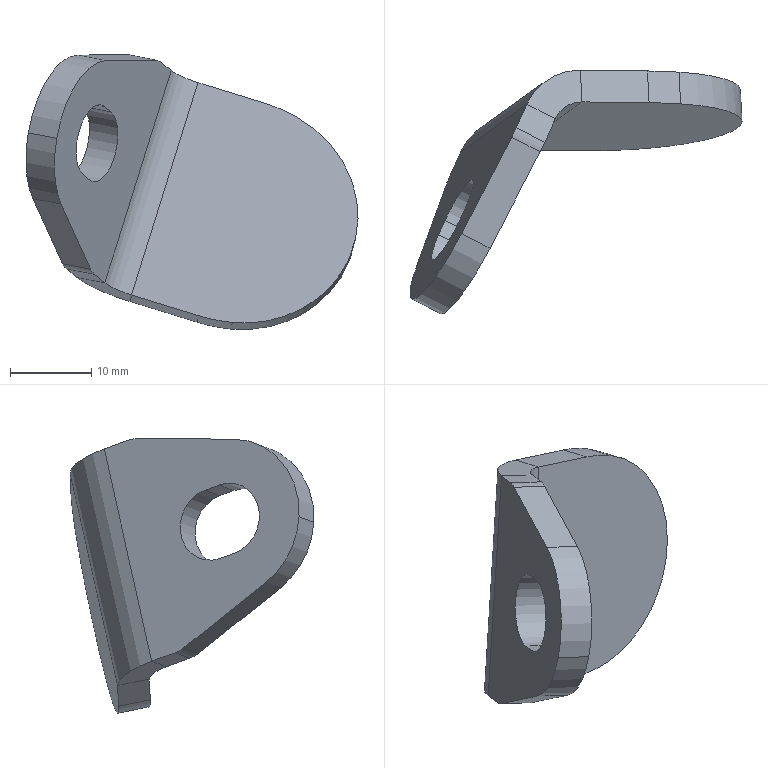Part | SolidWorks | features BaseBody 1 | 1 solid | 26 faces | box 40.878 x 30.009 x 33.842 mm | volume 4842 mm3 | plane 14 | cylinder 10 | spline 2 | commonest cylinder face diameters 8 x3 9 x2 20 x2 40 x2 16 x1
STEP:
#1=CARTESIAN_POINT('',(-7.748,15.098,8.963));
#2=VERTEX_POINT('',#1);
#3=CARTESIAN_POINT('',(-5.124,16.976,17.364));
#4=VERTEX_POINT('',#3);
#5=CARTESIAN_POINT('',(-6.436,16.037,13.163));
#6=DIRECTION('',(-0.8743,0.454,0.1717));
#7=DIRECTION('',(-0.2916,-0.2086,-0.9335));
#8=AXIS2_PLACEMENT_3D('',#5,#6,#7);
#9=CIRCLE('',#8,4.5);
#10=EDGE_CURVE('',#2,#4,#9,.T.);
#11=ORIENTED_EDGE('',*,*,#10,.F.);
#12=CARTESIAN_POINT('',(-6.972,16.831,8.333));
#13=VERTEX_POINT('',#12);
#14=CARTESIAN_POINT('',(-6.972,16.831,8.333));
#15=DIRECTION('',(-0.388,-0.8662,0.3148));
#16=VECTOR('',#15,1000.);
#17=LINE('',#14,#16);
#18=EDGE_CURVE('',#13,#2,#17,.T.);
#19=ORIENTED_EDGE('',*,*,#18,.F.);
#20=CARTESIAN_POINT('',(-4.348,18.709,16.734));
#21=VERTEX_POINT('',#20);
#22=CARTESIAN_POINT('',(-5.66,17.77,12.534));
#23=DIRECTION('',(-0.8743,0.454,0.1717));
#24=DIRECTION('',(0.2916,0.2086,0.9335));
#25=AXIS2_PLACEMENT_3D('',#22,#23,#24);
#26=CIRCLE('',#25,4.5);
#27=EDGE_CURVE('',#21,#13,#26,.T.);
#28=ORIENTED_EDGE('',*,*,#27,.F.);
#29=CARTESIAN_POINT('',(-5.124,16.976,17.364));
#30=DIRECTION('',(0.388,0.8662,-0.3148));
#31=VECTOR('',#30,1000.);
#32=LINE('',#29,#31);
#33=EDGE_CURVE('',#4,#21,#32,.T.);
#34=ORIENTED_EDGE('',*,*,#33,.F.);
#35=EDGE_LOOP('',(#11,#19,#28,#34));
#36=FACE_BOUND('',#35,.T.);
#37=CARTESIAN_POINT('',(3.098,31.128,21.809));
#38=VERTEX_POINT('',#37);
#39=CARTESIAN_POINT('',(1.803,28.238,22.859));
#40=VERTEX_POINT('',#39);
#41=CARTESIAN_POINT('',(3.098,31.128,21.809));
#42=DIRECTION('',(-0.388,-0.8662,0.3148));
#43=VECTOR('',#42,1000.);
#44=LINE('',#41,#43);
#45=EDGE_CURVE('',#38,#40,#44,.T.);
#46=ORIENTED_EDGE('',*,*,#45,.F.);
#47=CARTESIAN_POINT('',(-5.068,25.286,-4.329));
#48=VERTEX_POINT('',#47);
#49=CARTESIAN_POINT('',(-5.068,25.286,-4.329));
#50=DIRECTION('',(0.2916,0.2086,0.9335));
#51=VECTOR('',#50,1000.);
#52=LINE('',#49,#51);
#53=EDGE_CURVE('',#48,#38,#52,.T.);
#54=ORIENTED_EDGE('',*,*,#53,.F.);
#55=CARTESIAN_POINT('',(-6.362,22.396,-3.278));
#56=VERTEX_POINT('',#55);
#57=CARTESIAN_POINT('',(-6.362,22.396,-3.278));
#58=DIRECTION('',(0.388,0.8662,-0.3148));
#59=VECTOR('',#58,1000.);
#60=LINE('',#57,#59);
#61=EDGE_CURVE('',#56,#48,#60,.T.);
#62=ORIENTED_EDGE('',*,*,#61,.F.);
#63=CARTESIAN_POINT('',(-6.801,21.321,-2.671));
#64=VERTEX_POINT('',#63);
#65=CARTESIAN_POINT('',(-5.196,23.231,0.4555));
#66=DIRECTION('',(0.8743,-0.454,-0.1717));
#67=DIRECTION('',(-0.4014,-0.4775,-0.7816));
#68=AXIS2_PLACEMENT_3D('',#65,#66,#67);
#69=CIRCLE('',#68,4.);
#70=EDGE_CURVE('',#64,#56,#69,.T.);
#71=ORIENTED_EDGE('',*,*,#70,.F.);
#72=CARTESIAN_POINT('',(-10.45,11.263,5.347));
#73=VERTEX_POINT('',#72);
#74=CARTESIAN_POINT('',(-10.45,11.263,5.347));
#75=DIRECTION('',(0.2729,0.7523,-0.5997));
#76=VECTOR('',#75,1000.);
#77=LINE('',#74,#76);
#78=EDGE_CURVE('',#73,#64,#77,.T.);
#79=ORIENTED_EDGE('',*,*,#78,.F.);
#80=CARTESIAN_POINT('',(-10.998,7.143,13.448));
#81=VERTEX_POINT('',#80);
#82=CARTESIAN_POINT('',(-6.436,16.037,13.163));
#83=DIRECTION('',(0.8743,-0.454,-0.1717));
#84=DIRECTION('',(-0.4562,-0.8894,0.02851));
#85=AXIS2_PLACEMENT_3D('',#82,#83,#84);
#86=CIRCLE('',#85,10.);
#87=EDGE_CURVE('',#81,#73,#86,.T.);
#88=ORIENTED_EDGE('',*,*,#87,.F.);
#89=CARTESIAN_POINT('',(-4.93,15.211,23.015));
#90=VERTEX_POINT('',#89);
#91=CARTESIAN_POINT('',(-6.436,16.037,13.163));
#92=DIRECTION('',(0.8743,-0.454,-0.1717));
#93=DIRECTION('',(-0.4562,-0.8894,0.02851));
#94=AXIS2_PLACEMENT_3D('',#91,#92,#93);
#95=CIRCLE('',#94,10.);
#96=EDGE_CURVE('',#90,#81,#95,.T.);
#97=ORIENTED_EDGE('',*,*,#96,.F.);
#98=CARTESIAN_POINT('',(1.239,27.073,23.066));
#99=VERTEX_POINT('',#98);
#100=CARTESIAN_POINT('',(1.239,27.073,23.066));
#101=DIRECTION('',(-0.4614,-0.8872,-0.003841));
#102=VECTOR('',#101,1000.);
#103=LINE('',#100,#102);
#104=EDGE_CURVE('',#99,#90,#103,.T.);
#105=ORIENTED_EDGE('',*,*,#104,.F.);
#106=CARTESIAN_POINT('',(0.6369,27.404,19.125));
#107=DIRECTION('',(0.8743,-0.454,-0.1717));
#108=DIRECTION('',(0.2916,0.2086,0.9335));
#109=AXIS2_PLACEMENT_3D('',#106,#107,#108);
#110=CIRCLE('',#109,4.);
#111=EDGE_CURVE('',#40,#99,#110,.T.);
#112=ORIENTED_EDGE('',*,*,#111,.F.);
#113=EDGE_LOOP('',(#46,#54,#62,#71,#79,#88,#97,#105,#112));
#114=FACE_OUTER_BOUND('',#113,.T.);
#115=CARTESIAN_POINT('',(101.216,-68.081,783.905));
#116=DIRECTION('',(-0.8743,0.454,0.1717));
#117=DIRECTION('',(0.1927,0.,0.9813));
#118=AXIS2_PLACEMENT_3D('',#115,#116,#117);
#119=PLANE('',#118);
#120=ADVANCED_FACE('',(#36,#114),#119,.T.);
#121=CARTESIAN_POINT('',(5.301,26.422,22.173));
#122=VERTEX_POINT('',#121);
#123=CARTESIAN_POINT('',(1.803,28.238,22.859));
#124=DIRECTION('',(0.8743,-0.454,-0.1717));
#125=VECTOR('',#124,1000.);
#126=LINE('',#123,#125);
#127=EDGE_CURVE('',#40,#122,#126,.T.);
#128=ORIENTED_EDGE('',*,*,#127,.F.);
#129=ORIENTED_EDGE('',*,*,#111,.T.);
#130=CARTESIAN_POINT('',(4.736,25.257,22.379));
#131=VERTEX_POINT('',#130);
#132=CARTESIAN_POINT('',(4.736,25.257,22.379));
#133=DIRECTION('',(-0.8743,0.454,0.1717));
#134=VECTOR('',#133,1000.);
#135=LINE('',#132,#134);
#136=EDGE_CURVE('',#131,#99,#135,.T.);
#137=ORIENTED_EDGE('',*,*,#136,.F.);
#138=CARTESIAN_POINT('',(4.134,25.588,18.439));
#139=DIRECTION('',(-0.8743,0.454,0.1717));
#140=DIRECTION('',(0.1506,-0.08257,0.9851));
#141=AXIS2_PLACEMENT_3D('',#138,#139,#140);
#142=CIRCLE('',#141,4.);
#143=EDGE_CURVE('',#131,#122,#142,.T.);
#144=ORIENTED_EDGE('',*,*,#143,.T.);
#145=EDGE_LOOP('',(#128,#129,#137,#144));
#146=FACE_OUTER_BOUND('',#145,.T.);
#147=CARTESIAN_POINT('',(-83.852,71.275,35.714));
#148=DIRECTION('',(0.8743,-0.454,-0.1717));
#149=DIRECTION('',(0.2916,0.2086,0.9335));
#150=AXIS2_PLACEMENT_3D('',#147,#148,#149);
#151=CYLINDRICAL_SURFACE('',#150,4.);
#152=ADVANCED_FACE('',(#146),#151,.T.);
#153=CARTESIAN_POINT('',(-3.475,15.015,7.646));
#154=VERTEX_POINT('',#153);
#155=CARTESIAN_POINT('',(-0.8504,16.893,16.048));
#156=VERTEX_POINT('',#155);
#157=CARTESIAN_POINT('',(-2.163,15.954,11.847));
#158=DIRECTION('',(0.8743,-0.454,-0.1717));
#159=DIRECTION('',(-0.2916,-0.2086,-0.9335));
#160=AXIS2_PLACEMENT_3D('',#157,#158,#159);
#161=CIRCLE('',#160,4.5);
#162=EDGE_CURVE('',#154,#156,#161,.T.);
#163=ORIENTED_EDGE('',*,*,#162,.F.);
#164=CARTESIAN_POINT('',(-4.251,13.282,8.276));
#165=VERTEX_POINT('',#164);
#166=CARTESIAN_POINT('',(-4.251,13.282,8.276));
#167=DIRECTION('',(0.388,0.8662,-0.3148));
#168=VECTOR('',#167,1000.);
#169=LINE('',#166,#168);
#170=EDGE_CURVE('',#165,#154,#169,.T.);
#171=ORIENTED_EDGE('',*,*,#170,.F.);
#172=CARTESIAN_POINT('',(-1.626,15.16,16.677));
#173=VERTEX_POINT('',#172);
#174=CARTESIAN_POINT('',(-2.939,14.221,12.477));
#175=DIRECTION('',(0.8743,-0.454,-0.1717));
#176=DIRECTION('',(0.2916,0.2086,0.9335));
#177=AXIS2_PLACEMENT_3D('',#174,#175,#176);
#178=CIRCLE('',#177,4.5);
#179=EDGE_CURVE('',#173,#165,#178,.T.);
#180=ORIENTED_EDGE('',*,*,#179,.F.);
#181=CARTESIAN_POINT('',(-0.8504,16.893,16.048));
#182=DIRECTION('',(-0.388,-0.8662,0.3148));
#183=VECTOR('',#182,1000.);
#184=LINE('',#181,#183);
#185=EDGE_CURVE('',#156,#173,#184,.T.);
#186=ORIENTED_EDGE('',*,*,#185,.F.);
#187=EDGE_LOOP('',(#163,#171,#180,#186));
#188=FACE_BOUND('',#187,.T.);
#189=CARTESIAN_POINT('',(-1.433,13.396,22.328));
#190=VERTEX_POINT('',#189);
#191=CARTESIAN_POINT('',(-1.433,13.396,22.328));
#192=DIRECTION('',(0.4614,0.8872,0.003841));
#193=VECTOR('',#192,1000.);
#194=LINE('',#191,#193);
#195=EDGE_CURVE('',#190,#131,#194,.T.);
#196=ORIENTED_EDGE('',*,*,#195,.F.);
#197=CARTESIAN_POINT('',(-7.501,5.327,12.762));
#198=VERTEX_POINT('',#197);
#199=CARTESIAN_POINT('',(-2.939,14.221,12.477));
#200=DIRECTION('',(-0.8743,0.454,0.1717));
#201=DIRECTION('',(-0.4562,-0.8894,0.02851));
#202=AXIS2_PLACEMENT_3D('',#199,#200,#201);
#203=CIRCLE('',#202,10.);
#204=EDGE_CURVE('',#198,#190,#203,.T.);
#205=ORIENTED_EDGE('',*,*,#204,.F.);
#206=CARTESIAN_POINT('',(-6.953,9.447,4.66));
#207=VERTEX_POINT('',#206);
#208=CARTESIAN_POINT('',(-2.939,14.221,12.477));
#209=DIRECTION('',(-0.8743,0.454,0.1717));
#210=DIRECTION('',(-0.4562,-0.8894,0.02851));
#211=AXIS2_PLACEMENT_3D('',#208,#209,#210);
#212=CIRCLE('',#211,10.);
#213=EDGE_CURVE('',#207,#198,#212,.T.);
#214=ORIENTED_EDGE('',*,*,#213,.F.);
#215=CARTESIAN_POINT('',(-3.304,19.505,-3.358));
#216=VERTEX_POINT('',#215);
#217=CARTESIAN_POINT('',(-3.304,19.505,-3.358));
#218=DIRECTION('',(-0.2729,-0.7523,0.5997));
#219=VECTOR('',#218,1000.);
#220=LINE('',#217,#219);
#221=EDGE_CURVE('',#216,#207,#220,.T.);
#222=ORIENTED_EDGE('',*,*,#221,.F.);
#223=CARTESIAN_POINT('',(-2.865,20.58,-3.965));
#224=VERTEX_POINT('',#223);
#225=CARTESIAN_POINT('',(-1.698,21.415,-0.2311));
#226=DIRECTION('',(-0.8743,0.454,0.1717));
#227=DIRECTION('',(-0.2916,-0.2086,-0.9335));
#228=AXIS2_PLACEMENT_3D('',#225,#226,#227);
#229=CIRCLE('',#228,4.);
#230=EDGE_CURVE('',#224,#216,#229,.T.);
#231=ORIENTED_EDGE('',*,*,#230,.F.);
#232=CARTESIAN_POINT('',(-1.571,23.47,-5.015));
#233=VERTEX_POINT('',#232);
#234=CARTESIAN_POINT('',(-1.571,23.47,-5.015));
#235=DIRECTION('',(-0.388,-0.8662,0.3148));
#236=VECTOR('',#235,1000.);
#237=LINE('',#234,#236);
#238=EDGE_CURVE('',#233,#224,#237,.T.);
#239=ORIENTED_EDGE('',*,*,#238,.F.);
#240=CARTESIAN_POINT('',(6.595,29.312,21.123));
#241=VERTEX_POINT('',#240);
#242=CARTESIAN_POINT('',(6.595,29.312,21.123));
#243=DIRECTION('',(-0.2916,-0.2086,-0.9335));
#244=VECTOR('',#243,1000.);
#245=LINE('',#242,#244);
#246=EDGE_CURVE('',#241,#233,#245,.T.);
#247=ORIENTED_EDGE('',*,*,#246,.F.);
#248=CARTESIAN_POINT('',(5.301,26.422,22.173));
#249=DIRECTION('',(0.388,0.8662,-0.3148));
#250=VECTOR('',#249,1000.);
#251=LINE('',#248,#250);
#252=EDGE_CURVE('',#122,#241,#251,.T.);
#253=ORIENTED_EDGE('',*,*,#252,.F.);
#254=ORIENTED_EDGE('',*,*,#143,.F.);
#255=EDGE_LOOP('',(#196,#205,#214,#222,#231,#239,#247,#253,#254));
#256=FACE_OUTER_BOUND('',#255,.T.);
#257=CARTESIAN_POINT('',(104.713,-69.897,783.219));
#258=DIRECTION('',(-0.8743,0.454,0.1717));
#259=DIRECTION('',(0.1927,0.,0.9813));
#260=AXIS2_PLACEMENT_3D('',#257,#258,#259);
#261=PLANE('',#260);
#262=ADVANCED_FACE('',(#188,#256),#261,.F.);
#263=ORIENTED_EDGE('',*,*,#252,.T.);
#264=CARTESIAN_POINT('',(6.595,29.312,21.123));
#265=DIRECTION('',(-0.8743,0.454,0.1717));
#266=VECTOR('',#265,1000.);
#267=LINE('',#264,#266);
#268=EDGE_CURVE('',#241,#38,#267,.T.);
#269=ORIENTED_EDGE('',*,*,#268,.T.);
#270=ORIENTED_EDGE('',*,*,#45,.T.);
#271=ORIENTED_EDGE('',*,*,#127,.T.);
#272=EDGE_LOOP('',(#263,#269,#270,#271));
#273=FACE_OUTER_BOUND('',#272,.T.);
#274=CARTESIAN_POINT('',(-2.695,13.384,27.585));
#275=DIRECTION('',(-0.2916,-0.2086,-0.9335));
#276=DIRECTION('',(-0.9545,0.,0.2982));
#277=AXIS2_PLACEMENT_3D('',#274,#275,#276);
#278=PLANE('',#277);
#279=ADVANCED_FACE('',(#273),#278,.F.);
#280=ORIENTED_EDGE('',*,*,#268,.F.);
#281=CARTESIAN_POINT('',(9.887,31.408,19.626));
#282=VERTEX_POINT('',#281);
#283=CARTESIAN_POINT('',(10.092,27.496,20.436));
#284=DIRECTION('',(0.2916,0.2086,0.9335));
#285=DIRECTION('',(-0.05124,0.9779,-0.2026));
#286=AXIS2_PLACEMENT_3D('',#283,#284,#285);
#287=CIRCLE('',#286,4.);
#288=EDGE_CURVE('',#282,#241,#287,.T.);
#289=ORIENTED_EDGE('',*,*,#288,.F.);
#290=CARTESIAN_POINT('',(9.682,35.319,18.815));
#291=VERTEX_POINT('',#290);
#292=CARTESIAN_POINT('',(9.887,31.408,19.626));
#293=DIRECTION('',(-0.05124,0.9779,-0.2026));
#294=VECTOR('',#293,1000.);
#295=LINE('',#292,#294);
#296=EDGE_CURVE('',#282,#291,#295,.T.);
#297=ORIENTED_EDGE('',*,*,#296,.T.);
#298=CARTESIAN_POINT('',(10.092,27.496,20.436));
#299=DIRECTION('',(-0.2916,-0.2086,-0.9335));
#300=DIRECTION('',(-0.8743,0.454,0.1717));
#301=AXIS2_PLACEMENT_3D('',#298,#299,#300);
#302=CIRCLE('',#301,8.);
#303=EDGE_CURVE('',#38,#291,#302,.T.);
#304=ORIENTED_EDGE('',*,*,#303,.F.);
#305=EDGE_LOOP('',(#280,#289,#297,#304));
#306=FACE_OUTER_BOUND('',#305,.T.);
#307=CARTESIAN_POINT('',(6.836,32.534,20.327));
#308=DIRECTION('',(-0.2916,-0.2086,-0.9335));
#309=DIRECTION('',(-0.9545,0.,0.2982));
#310=AXIS2_PLACEMENT_3D('',#307,#308,#309);
#311=PLANE('',#310);
#312=ADVANCED_FACE('',(#306),#311,.F.);
#313=CARTESIAN_POINT('',(1.517,29.477,-7.323));
#314=VERTEX_POINT('',#313);
#315=CARTESIAN_POINT('',(1.926,21.654,-5.702));
#316=DIRECTION('',(0.2916,0.2086,0.9335));
#317=DIRECTION('',(-0.05124,0.9779,-0.2026));
#318=AXIS2_PLACEMENT_3D('',#315,#316,#317);
#319=CIRCLE('',#318,8.);
#320=EDGE_CURVE('',#314,#48,#319,.T.);
#321=ORIENTED_EDGE('',*,*,#320,.T.);
#322=ORIENTED_EDGE('',*,*,#53,.T.);
#323=ORIENTED_EDGE('',*,*,#303,.T.);
#324=CARTESIAN_POINT('',(1.517,29.477,-7.323));
#325=DIRECTION('',(0.2916,0.2086,0.9335));
#326=VECTOR('',#325,1000.);
#327=LINE('',#324,#326);
#328=EDGE_CURVE('',#314,#291,#327,.T.);
#329=ORIENTED_EDGE('',*,*,#328,.F.);
#330=EDGE_LOOP('',(#321,#322,#323,#329));
#331=FACE_OUTER_BOUND('',#330,.T.);
#332=CARTESIAN_POINT('',(49.385,55.609,146.213));
#333=DIRECTION('',(-0.2916,-0.2086,-0.9335));
#334=DIRECTION('',(-0.8743,0.454,0.1717));
#335=AXIS2_PLACEMENT_3D('',#332,#333,#334);
#336=CYLINDRICAL_SURFACE('',#335,8.);
#337=ADVANCED_FACE('',(#331),#336,.T.);
#338=CARTESIAN_POINT('',(9.775,29.38,-9.881));
#339=VERTEX_POINT('',#338);
#340=CARTESIAN_POINT('',(13.921,29.426,-10.708));
#341=VERTEX_POINT('',#340);
#342=CARTESIAN_POINT('',(15.608,33.553,8.789));
#343=DIRECTION('',(0.05124,-0.9779,0.2026));
#344=DIRECTION('',(-0.2916,-0.2086,-0.9335));
#345=AXIS2_PLACEMENT_3D('',#342,#343,#344);
#346=CIRCLE('',#345,20.);
#347=EDGE_CURVE('',#339,#341,#346,.T.);
#348=ORIENTED_EDGE('',*,*,#347,.F.);
#349=CARTESIAN_POINT('',(9.775,29.38,-9.881));
#350=DIRECTION('',(-0.9552,0.01125,0.2959));
#351=VECTOR('',#350,1000.);
#352=LINE('',#349,#351);
#353=EDGE_CURVE('',#339,#314,#352,.T.);
#354=ORIENTED_EDGE('',*,*,#353,.T.);
#355=ORIENTED_EDGE('',*,*,#328,.T.);
#356=CARTESIAN_POINT('',(17.943,35.222,16.256));
#357=VERTEX_POINT('',#356);
#358=CARTESIAN_POINT('',(17.943,35.222,16.256));
#359=DIRECTION('',(-0.9552,0.01125,0.2959));
#360=VECTOR('',#359,1000.);
#361=LINE('',#358,#360);
#362=EDGE_CURVE('',#357,#291,#361,.T.);
#363=ORIENTED_EDGE('',*,*,#362,.F.);
#364=CARTESIAN_POINT('',(21.827,35.082,14.596));
#365=VERTEX_POINT('',#364);
#366=CARTESIAN_POINT('',(12.11,31.049,-2.414));
#367=DIRECTION('',(0.05124,-0.9779,0.2026));
#368=DIRECTION('',(0.4858,0.2016,0.8505));
#369=AXIS2_PLACEMENT_3D('',#366,#367,#368);
#370=CIRCLE('',#369,20.);
#371=EDGE_CURVE('',#365,#357,#370,.T.);
#372=ORIENTED_EDGE('',*,*,#371,.F.);
#373=CARTESIAN_POINT('',(24.496,30.606,-7.683));
#374=VERTEX_POINT('',#373);
#375=CARTESIAN_POINT('',(24.496,30.606,-7.683));
#376=CARTESIAN_POINT('',(25.008,30.717,-7.276));
#377=CARTESIAN_POINT('',(25.954,30.947,-6.406));
#378=CARTESIAN_POINT('',(27.159,31.318,-4.919));
#379=CARTESIAN_POINT('',(28.114,31.703,-3.303));
#380=CARTESIAN_POINT('',(28.823,32.102,-1.558));
#381=CARTESIAN_POINT('',(29.261,32.5,0.2521));
#382=CARTESIAN_POINT('',(29.429,32.899,2.136));
#383=CARTESIAN_POINT('',(29.317,33.285,4.027));
#384=CARTESIAN_POINT('',(28.923,33.656,5.921));
#385=CARTESIAN_POINT('',(28.247,34.003,7.768));
#386=CARTESIAN_POINT('',(27.298,34.319,9.532));
#387=CARTESIAN_POINT('',(26.079,34.598,11.186));
#388=CARTESIAN_POINT('',(24.623,34.83,12.672));
#389=CARTESIAN_POINT('',(23.165,34.987,13.799));
#390=CARTESIAN_POINT('',(22.197,35.058,14.39));
#391=CARTESIAN_POINT('',(21.827,35.082,14.596));
#392=B_SPLINE_CURVE_WITH_KNOTS('',3,(#375,#376,#377,#378,#379,#380,#381,#382,#383,#384,#385,#386,#387,#388,#389,#390,#391),.UNSPECIFIED.,.F.,.F.,(4,1,1,1,1,1,1,1,1,1,1,1,1,1,4),(0.,0.07356,0.1471,0.2207,0.2943,0.3678,0.4414,0.5149,0.5885,0.6621,0.7356,0.8092,0.8828,0.9563,1.),.UNSPECIFIED.);
#393=EDGE_CURVE('',#374,#365,#392,.T.);
#394=ORIENTED_EDGE('',*,*,#393,.F.);
#395=CARTESIAN_POINT('',(13.921,29.426,-10.708));
#396=CARTESIAN_POINT('',(14.299,29.438,-10.743));
#397=CARTESIAN_POINT('',(15.386,29.482,-10.805));
#398=CARTESIAN_POINT('',(17.155,29.592,-10.722));
#399=CARTESIAN_POINT('',(19.202,29.778,-10.344));
#400=CARTESIAN_POINT('',(21.126,30.011,-9.705));
#401=CARTESIAN_POINT('',(22.923,30.289,-8.815));
#402=CARTESIAN_POINT('',(23.99,30.497,-8.084));
#403=CARTESIAN_POINT('',(24.496,30.606,-7.683));
#404=B_SPLINE_CURVE_WITH_KNOTS('',3,(#395,#396,#397,#398,#399,#400,#401,#402,#403),.UNSPECIFIED.,.F.,.F.,(4,1,1,1,1,1,4),(0.,0.0968,0.2774,0.4581,0.6387,0.8194,1.),.UNSPECIFIED.);
#405=EDGE_CURVE('',#341,#374,#404,.T.);
#406=ORIENTED_EDGE('',*,*,#405,.F.);
#407=EDGE_LOOP('',(#348,#354,#355,#363,#372,#394,#406));
#408=FACE_OUTER_BOUND('',#407,.T.);
#409=CARTESIAN_POINT('',(21.358,32.213,0.8648));
#410=DIRECTION('',(-0.05124,0.9779,-0.2026));
#411=DIRECTION('',(-0.9695,0.,0.2452));
#412=AXIS2_PLACEMENT_3D('',#409,#410,#411);
#413=PLANE('',#412);
#414=ADVANCED_FACE('',(#408),#413,.T.);
#415=CARTESIAN_POINT('',(24.701,26.695,-6.872));
#416=VERTEX_POINT('',#415);
#417=CARTESIAN_POINT('',(24.701,26.695,-6.872));
#418=DIRECTION('',(-0.05124,0.9779,-0.2026));
#419=VECTOR('',#418,1000.);
#420=LINE('',#417,#419);
#421=EDGE_CURVE('',#416,#374,#420,.T.);
#422=ORIENTED_EDGE('',*,*,#421,.F.);
#423=CARTESIAN_POINT('',(14.126,25.514,-9.897));
#424=VERTEX_POINT('',#423);
#425=CARTESIAN_POINT('',(24.701,26.695,-6.872));
#426=CARTESIAN_POINT('',(24.195,26.585,-7.274));
#427=CARTESIAN_POINT('',(23.128,26.378,-8.005));
#428=CARTESIAN_POINT('',(21.331,26.099,-8.895));
#429=CARTESIAN_POINT('',(19.407,25.866,-9.533));
#430=CARTESIAN_POINT('',(17.36,25.68,-9.912));
#431=CARTESIAN_POINT('',(15.591,25.571,-9.995));
#432=CARTESIAN_POINT('',(14.504,25.527,-9.933));
#433=CARTESIAN_POINT('',(14.126,25.514,-9.897));
#434=B_SPLINE_CURVE_WITH_KNOTS('',3,(#425,#426,#427,#428,#429,#430,#431,#432,#433),.UNSPECIFIED.,.F.,.F.,(4,1,1,1,1,1,4),(0.,0.1806,0.3613,0.5419,0.7226,0.9032,1.),.UNSPECIFIED.);
#435=EDGE_CURVE('',#416,#424,#434,.T.);
#436=ORIENTED_EDGE('',*,*,#435,.T.);
#437=CARTESIAN_POINT('',(13.921,29.426,-10.708));
#438=DIRECTION('',(0.05124,-0.9779,0.2026));
#439=VECTOR('',#438,1000.);
#440=LINE('',#437,#439);
#441=EDGE_CURVE('',#341,#424,#440,.T.);
#442=ORIENTED_EDGE('',*,*,#441,.F.);
#443=ORIENTED_EDGE('',*,*,#405,.T.);
#444=EDGE_LOOP('',(#422,#436,#442,#443));
#445=FACE_OUTER_BOUND('',#444,.T.);
#446=CARTESIAN_POINT('',(24.701,26.695,-6.872));
#447=CARTESIAN_POINT('',(24.496,30.606,-7.683));
#448=CARTESIAN_POINT('',(24.195,26.585,-7.274));
#449=CARTESIAN_POINT('',(23.99,30.497,-8.084));
#450=CARTESIAN_POINT('',(23.128,26.378,-8.005));
#451=CARTESIAN_POINT('',(22.923,30.289,-8.815));
#452=CARTESIAN_POINT('',(21.331,26.099,-8.895));
#453=CARTESIAN_POINT('',(21.126,30.011,-9.705));
#454=CARTESIAN_POINT('',(19.407,25.866,-9.533));
#455=CARTESIAN_POINT('',(19.202,29.778,-10.344));
#456=CARTESIAN_POINT('',(17.36,25.68,-9.912));
#457=CARTESIAN_POINT('',(17.155,29.592,-10.722));
#458=CARTESIAN_POINT('',(15.591,25.571,-9.995));
#459=CARTESIAN_POINT('',(15.386,29.482,-10.805));
#460=CARTESIAN_POINT('',(14.504,25.527,-9.933));
#461=CARTESIAN_POINT('',(14.299,29.438,-10.743));
#462=CARTESIAN_POINT('',(14.126,25.514,-9.897));
#463=CARTESIAN_POINT('',(13.921,29.426,-10.708));
#464=B_SPLINE_SURFACE_WITH_KNOTS('',3,1,((#446,#447),(#448,#449),(#450,#451),(#452,#453),(#454,#455),(#456,#457),(#458,#459),(#460,#461),(#462,#463)),.UNSPECIFIED.,.F.,.F.,.F.,(4,1,1,1,1,1,4),(2,2),(0.01022,0.1873,0.3644,0.5415,0.7186,0.8957,0.9906),(0.,1.),.UNSPECIFIED.);
#465=ADVANCED_FACE('',(#445),#464,.T.);
#466=ORIENTED_EDGE('',*,*,#441,.T.);
#467=CARTESIAN_POINT('',(9.98,25.468,-9.07));
#468=VERTEX_POINT('',#467);
#469=CARTESIAN_POINT('',(15.813,29.641,9.599));
#470=DIRECTION('',(-0.05124,0.9779,-0.2026));
#471=DIRECTION('',(-0.08435,-0.2064,-0.9748));
#472=AXIS2_PLACEMENT_3D('',#469,#470,#471);
#473=CIRCLE('',#472,20.);
#474=EDGE_CURVE('',#424,#468,#473,.T.);
#475=ORIENTED_EDGE('',*,*,#474,.T.);
#476=CARTESIAN_POINT('',(9.775,29.38,-9.881));
#477=DIRECTION('',(0.05124,-0.9779,0.2026));
#478=VECTOR('',#477,1000.);
#479=LINE('',#476,#478);
#480=EDGE_CURVE('',#339,#468,#479,.T.);
#481=ORIENTED_EDGE('',*,*,#480,.F.);
#482=ORIENTED_EDGE('',*,*,#347,.T.);
#483=EDGE_LOOP('',(#466,#475,#481,#482));
#484=FACE_OUTER_BOUND('',#483,.T.);
#485=CARTESIAN_POINT('',(15.608,33.553,8.789));
#486=DIRECTION('',(-0.05124,0.9779,-0.2026));
#487=DIRECTION('',(-0.9987,-0.05017,0.01039));
#488=AXIS2_PLACEMENT_3D('',#485,#486,#487);
#489=CYLINDRICAL_SURFACE('',#488,20.);
#490=ADVANCED_FACE('',(#484),#489,.T.);
#491=CARTESIAN_POINT('',(1.721,25.565,-6.512));
#492=VERTEX_POINT('',#491);
#493=CARTESIAN_POINT('',(9.98,25.468,-9.07));
#494=DIRECTION('',(-0.9552,0.01125,0.2959));
#495=VECTOR('',#494,1000.);
#496=LINE('',#493,#495);
#497=EDGE_CURVE('',#468,#492,#496,.T.);
#498=ORIENTED_EDGE('',*,*,#497,.T.);
#499=CARTESIAN_POINT('',(1.721,25.565,-6.512));
#500=DIRECTION('',(-0.05124,0.9779,-0.2026));
#501=VECTOR('',#500,1000.);
#502=LINE('',#499,#501);
#503=EDGE_CURVE('',#492,#314,#502,.T.);
#504=ORIENTED_EDGE('',*,*,#503,.T.);
#505=ORIENTED_EDGE('',*,*,#353,.F.);
#506=ORIENTED_EDGE('',*,*,#480,.T.);
#507=EDGE_LOOP('',(#498,#504,#505,#506));
#508=FACE_OUTER_BOUND('',#507,.T.);
#509=CARTESIAN_POINT('',(16.793,27.343,-11.618));
#510=DIRECTION('',(0.2916,0.2086,0.9335));
#511=DIRECTION('',(0.5819,-0.8133,0.));
#512=AXIS2_PLACEMENT_3D('',#509,#510,#511);
#513=PLANE('',#512);
#514=ADVANCED_FACE('',(#508),#513,.F.);
#515=ORIENTED_EDGE('',*,*,#503,.F.);
#516=CARTESIAN_POINT('',(1.926,21.654,-5.702));
#517=DIRECTION('',(-0.2916,-0.2086,-0.9335));
#518=DIRECTION('',(-0.8743,0.454,0.1717));
#519=AXIS2_PLACEMENT_3D('',#516,#517,#518);
#520=CIRCLE('',#519,4.);
#521=EDGE_CURVE('',#233,#492,#520,.T.);
#522=ORIENTED_EDGE('',*,*,#521,.F.);
#523=CARTESIAN_POINT('',(-1.571,23.47,-5.015));
#524=DIRECTION('',(-0.8743,0.454,0.1717));
#525=VECTOR('',#524,1000.);
#526=LINE('',#523,#525);
#527=EDGE_CURVE('',#233,#48,#526,.T.);
#528=ORIENTED_EDGE('',*,*,#527,.T.);
#529=ORIENTED_EDGE('',*,*,#320,.F.);
#530=EDGE_LOOP('',(#515,#522,#528,#529));
#531=FACE_OUTER_BOUND('',#530,.T.);
#532=CARTESIAN_POINT('',(-1.33,26.692,-5.811));
#533=DIRECTION('',(0.2916,0.2086,0.9335));
#534=DIRECTION('',(0.5819,-0.8133,0.));
#535=AXIS2_PLACEMENT_3D('',#532,#533,#534);
#536=PLANE('',#535);
#537=ADVANCED_FACE('',(#531),#536,.F.);
#538=ORIENTED_EDGE('',*,*,#61,.T.);
#539=ORIENTED_EDGE('',*,*,#527,.F.);
#540=ORIENTED_EDGE('',*,*,#238,.T.);
#541=CARTESIAN_POINT('',(-2.865,20.58,-3.965));
#542=DIRECTION('',(-0.8743,0.454,0.1717));
#543=VECTOR('',#542,1000.);
#544=LINE('',#541,#543);
#545=EDGE_CURVE('',#224,#56,#544,.T.);
#546=ORIENTED_EDGE('',*,*,#545,.T.);
#547=EDGE_LOOP('',(#538,#539,#540,#546));
#548=FACE_OUTER_BOUND('',#547,.T.);
#549=CARTESIAN_POINT('',(-10.86,7.542,1.447));
#550=DIRECTION('',(0.2916,0.2086,0.9335));
#551=DIRECTION('',(0.5819,-0.8133,0.));
#552=AXIS2_PLACEMENT_3D('',#549,#550,#551);
#553=PLANE('',#552);
#554=ADVANCED_FACE('',(#548),#553,.F.);
#555=ORIENTED_EDGE('',*,*,#545,.F.);
#556=ORIENTED_EDGE('',*,*,#230,.T.);
#557=CARTESIAN_POINT('',(-6.801,21.321,-2.671));
#558=DIRECTION('',(0.8743,-0.454,-0.1717));
#559=VECTOR('',#558,1000.);
#560=LINE('',#557,#559);
#561=EDGE_CURVE('',#64,#216,#560,.T.);
#562=ORIENTED_EDGE('',*,*,#561,.F.);
#563=ORIENTED_EDGE('',*,*,#70,.T.);
#564=EDGE_LOOP('',(#555,#556,#562,#563));
#565=FACE_OUTER_BOUND('',#564,.T.);
#566=CARTESIAN_POINT('',(90.232,-26.32,-18.281));
#567=DIRECTION('',(-0.8743,0.454,0.1717));
#568=DIRECTION('',(-0.2916,-0.2086,-0.9335));
#569=AXIS2_PLACEMENT_3D('',#566,#567,#568);
#570=CYLINDRICAL_SURFACE('',#569,4.);
#571=ADVANCED_FACE('',(#565),#570,.T.);
#572=ORIENTED_EDGE('',*,*,#221,.T.);
#573=CARTESIAN_POINT('',(-6.953,9.447,4.66));
#574=DIRECTION('',(-0.8743,0.454,0.1717));
#575=VECTOR('',#574,1000.);
#576=LINE('',#573,#575);
#577=EDGE_CURVE('',#207,#73,#576,.T.);
#578=ORIENTED_EDGE('',*,*,#577,.T.);
#579=ORIENTED_EDGE('',*,*,#78,.T.);
#580=ORIENTED_EDGE('',*,*,#561,.T.);
#581=EDGE_LOOP('',(#572,#578,#579,#580));
#582=FACE_OUTER_BOUND('',#581,.T.);
#583=CARTESIAN_POINT('',(-10.45,11.263,5.347));
#584=DIRECTION('',(0.4014,0.4775,0.7816));
#585=DIRECTION('',(0.7655,-0.6435,0.));
#586=AXIS2_PLACEMENT_3D('',#583,#584,#585);
#587=PLANE('',#586);
#588=ADVANCED_FACE('',(#582),#587,.F.);
#589=CARTESIAN_POINT('',(-10.998,7.143,13.448));
#590=DIRECTION('',(-0.8743,0.454,0.1717));
#591=VECTOR('',#590,1000.);
#592=LINE('',#589,#591);
#593=EDGE_CURVE('',#198,#81,#592,.T.);
#594=ORIENTED_EDGE('',*,*,#593,.F.);
#595=ORIENTED_EDGE('',*,*,#204,.T.);
#596=CARTESIAN_POINT('',(-4.93,15.211,23.015));
#597=DIRECTION('',(0.8743,-0.454,-0.1717));
#598=VECTOR('',#597,1000.);
#599=LINE('',#596,#598);
#600=EDGE_CURVE('',#90,#190,#599,.T.);
#601=ORIENTED_EDGE('',*,*,#600,.F.);
#602=ORIENTED_EDGE('',*,*,#96,.T.);
#603=EDGE_LOOP('',(#594,#595,#601,#602));
#604=FACE_OUTER_BOUND('',#603,.T.);
#605=CARTESIAN_POINT('',(-6.436,16.037,13.163));
#606=DIRECTION('',(-0.8743,0.454,0.1717));
#607=DIRECTION('',(-0.4562,-0.8894,0.02851));
#608=AXIS2_PLACEMENT_3D('',#605,#606,#607);
#609=CYLINDRICAL_SURFACE('',#608,10.);
#610=ADVANCED_FACE('',(#604),#609,.T.);
#611=ORIENTED_EDGE('',*,*,#104,.T.);
#612=ORIENTED_EDGE('',*,*,#600,.T.);
#613=ORIENTED_EDGE('',*,*,#195,.T.);
#614=ORIENTED_EDGE('',*,*,#136,.T.);
#615=EDGE_LOOP('',(#611,#612,#613,#614));
#616=FACE_OUTER_BOUND('',#615,.T.);
#617=CARTESIAN_POINT('',(1.546,27.663,23.069));
#618=DIRECTION('',(-0.1506,0.08257,-0.9851));
#619=DIRECTION('',(-0.9885,0.,0.1511));
#620=AXIS2_PLACEMENT_3D('',#617,#618,#619);
#621=PLANE('',#620);
#622=ADVANCED_FACE('',(#616),#621,.F.);
#623=ORIENTED_EDGE('',*,*,#288,.T.);
#624=ORIENTED_EDGE('',*,*,#246,.T.);
#625=ORIENTED_EDGE('',*,*,#521,.T.);
#626=CARTESIAN_POINT('',(9.887,31.408,19.626));
#627=DIRECTION('',(-0.2916,-0.2086,-0.9335));
#628=VECTOR('',#627,1000.);
#629=LINE('',#626,#628);
#630=EDGE_CURVE('',#282,#492,#629,.T.);
#631=ORIENTED_EDGE('',*,*,#630,.F.);
#632=EDGE_LOOP('',(#623,#624,#625,#631));
#633=FACE_OUTER_BOUND('',#632,.T.);
#634=CARTESIAN_POINT('',(49.385,55.609,146.213));
#635=DIRECTION('',(-0.2916,-0.2086,-0.9335));
#636=DIRECTION('',(-0.8743,0.454,0.1717));
#637=AXIS2_PLACEMENT_3D('',#634,#635,#636);
#638=CYLINDRICAL_SURFACE('',#637,4.);
#639=ADVANCED_FACE('',(#633),#638,.F.);
#640=CARTESIAN_POINT('',(22.032,31.17,15.406));
#641=VERTEX_POINT('',#640);
#642=CARTESIAN_POINT('',(22.032,31.17,15.406));
#643=CARTESIAN_POINT('',(22.402,31.147,15.201));
#644=CARTESIAN_POINT('',(23.37,31.075,14.609));
#645=CARTESIAN_POINT('',(24.828,30.918,13.483));
#646=CARTESIAN_POINT('',(26.284,30.686,11.996));
#647=CARTESIAN_POINT('',(27.503,30.407,10.342));
#648=CARTESIAN_POINT('',(28.452,30.092,8.578));
#649=CARTESIAN_POINT('',(29.128,29.745,6.731));
#650=CARTESIAN_POINT('',(29.522,29.373,4.838));
#651=CARTESIAN_POINT('',(29.634,28.987,2.946));
#652=CARTESIAN_POINT('',(29.466,28.588,1.062));
#653=CARTESIAN_POINT('',(29.028,28.19,-0.7476));
#654=CARTESIAN_POINT('',(28.319,27.791,-2.493));
#655=CARTESIAN_POINT('',(27.364,27.407,-4.108));
#656=CARTESIAN_POINT('',(26.159,27.036,-5.595));
#657=CARTESIAN_POINT('',(25.213,26.806,-6.466));
#658=CARTESIAN_POINT('',(24.701,26.695,-6.872));
#659=B_SPLINE_CURVE_WITH_KNOTS('',3,(#642,#643,#644,#645,#646,#647,#648,#649,#650,#651,#652,#653,#654,#655,#656,#657,#658),.UNSPECIFIED.,.F.,.F.,(4,1,1,1,1,1,1,1,1,1,1,1,1,1,4),(0.,0.04368,0.1172,0.1908,0.2644,0.3379,0.4115,0.4851,0.5586,0.6322,0.7057,0.7793,0.8529,0.9264,1.),.UNSPECIFIED.);
#660=EDGE_CURVE('',#641,#416,#659,.T.);
#661=ORIENTED_EDGE('',*,*,#660,.F.);
#662=CARTESIAN_POINT('',(18.148,31.31,17.067));
#663=VERTEX_POINT('',#662);
#664=CARTESIAN_POINT('',(12.315,27.137,-1.603));
#665=DIRECTION('',(-0.05124,0.9779,-0.2026));
#666=DIRECTION('',(0.2916,0.2086,0.9335));
#667=AXIS2_PLACEMENT_3D('',#664,#665,#666);
#668=CIRCLE('',#667,20.);
#669=EDGE_CURVE('',#663,#641,#668,.T.);
#670=ORIENTED_EDGE('',*,*,#669,.F.);
#671=CARTESIAN_POINT('',(18.148,31.31,17.067));
#672=DIRECTION('',(-0.9552,0.01125,0.2959));
#673=VECTOR('',#672,1000.);
#674=LINE('',#671,#673);
#675=EDGE_CURVE('',#663,#282,#674,.T.);
#676=ORIENTED_EDGE('',*,*,#675,.T.);
#677=ORIENTED_EDGE('',*,*,#630,.T.);
#678=ORIENTED_EDGE('',*,*,#497,.F.);
#679=ORIENTED_EDGE('',*,*,#474,.F.);
#680=ORIENTED_EDGE('',*,*,#435,.F.);
#681=EDGE_LOOP('',(#661,#670,#676,#677,#678,#679,#680));
#682=FACE_OUTER_BOUND('',#681,.T.);
#683=CARTESIAN_POINT('',(21.563,28.301,1.675));
#684=DIRECTION('',(-0.05124,0.9779,-0.2026));
#685=DIRECTION('',(-0.9695,0.,0.2452));
#686=AXIS2_PLACEMENT_3D('',#683,#684,#685);
#687=PLANE('',#686);
#688=ADVANCED_FACE('',(#682),#687,.F.);
#689=ORIENTED_EDGE('',*,*,#296,.F.);
#690=ORIENTED_EDGE('',*,*,#675,.F.);
#691=CARTESIAN_POINT('',(18.148,31.31,17.067));
#692=DIRECTION('',(-0.05124,0.9779,-0.2026));
#693=VECTOR('',#692,1000.);
#694=LINE('',#691,#693);
#695=EDGE_CURVE('',#663,#357,#694,.T.);
#696=ORIENTED_EDGE('',*,*,#695,.T.);
#697=ORIENTED_EDGE('',*,*,#362,.T.);
#698=EDGE_LOOP('',(#689,#690,#696,#697));
#699=FACE_OUTER_BOUND('',#698,.T.);
#700=CARTESIAN_POINT('',(24.958,33.185,14.52));
#701=DIRECTION('',(0.2916,0.2086,0.9335));
#702=DIRECTION('',(0.5819,-0.8133,0.));
#703=AXIS2_PLACEMENT_3D('',#700,#701,#702);
#704=PLANE('',#703);
#705=ADVANCED_FACE('',(#699),#704,.T.);
#706=ORIENTED_EDGE('',*,*,#695,.F.);
#707=ORIENTED_EDGE('',*,*,#669,.T.);
#708=CARTESIAN_POINT('',(22.032,31.17,15.406));
#709=DIRECTION('',(-0.05124,0.9779,-0.2026));
#710=VECTOR('',#709,1000.);
#711=LINE('',#708,#710);
#712=EDGE_CURVE('',#641,#365,#711,.T.);
#713=ORIENTED_EDGE('',*,*,#712,.T.);
#714=ORIENTED_EDGE('',*,*,#371,.T.);
#715=EDGE_LOOP('',(#706,#707,#713,#714));
#716=FACE_OUTER_BOUND('',#715,.T.);
#717=CARTESIAN_POINT('',(12.11,31.049,-2.414));
#718=DIRECTION('',(-0.05124,0.9779,-0.2026));
#719=DIRECTION('',(-0.9987,-0.05017,0.01039));
#720=AXIS2_PLACEMENT_3D('',#717,#718,#719);
#721=CYLINDRICAL_SURFACE('',#720,20.);
#722=ADVANCED_FACE('',(#716),#721,.T.);
#723=ORIENTED_EDGE('',*,*,#712,.F.);
#724=ORIENTED_EDGE('',*,*,#660,.T.);
#725=ORIENTED_EDGE('',*,*,#421,.T.);
#726=ORIENTED_EDGE('',*,*,#393,.T.);
#727=EDGE_LOOP('',(#723,#724,#725,#726));
#728=FACE_OUTER_BOUND('',#727,.T.);
#729=CARTESIAN_POINT('',(22.032,31.17,15.406));
#730=CARTESIAN_POINT('',(21.827,35.082,14.596));
#731=CARTESIAN_POINT('',(22.402,31.147,15.201));
#732=CARTESIAN_POINT('',(22.197,35.058,14.39));
#733=CARTESIAN_POINT('',(23.37,31.075,14.609));
#734=CARTESIAN_POINT('',(23.165,34.987,13.799));
#735=CARTESIAN_POINT('',(24.828,30.918,13.483));
#736=CARTESIAN_POINT('',(24.623,34.83,12.672));
#737=CARTESIAN_POINT('',(26.284,30.686,11.996));
#738=CARTESIAN_POINT('',(26.079,34.598,11.186));
#739=CARTESIAN_POINT('',(27.503,30.407,10.342));
#740=CARTESIAN_POINT('',(27.298,34.319,9.532));
#741=CARTESIAN_POINT('',(28.452,30.092,8.578));
#742=CARTESIAN_POINT('',(28.247,34.003,7.768));
#743=CARTESIAN_POINT('',(29.128,29.745,6.731));
#744=CARTESIAN_POINT('',(28.923,33.656,5.921));
#745=CARTESIAN_POINT('',(29.522,29.373,4.838));
#746=CARTESIAN_POINT('',(29.317,33.285,4.027));
#747=CARTESIAN_POINT('',(29.634,28.987,2.946));
#748=CARTESIAN_POINT('',(29.429,32.899,2.136));
#749=CARTESIAN_POINT('',(29.466,28.588,1.062));
#750=CARTESIAN_POINT('',(29.261,32.5,0.2521));
#751=CARTESIAN_POINT('',(29.028,28.19,-0.7476));
#752=CARTESIAN_POINT('',(28.823,32.102,-1.558));
#753=CARTESIAN_POINT('',(28.319,27.791,-2.493));
#754=CARTESIAN_POINT('',(28.114,31.703,-3.303));
#755=CARTESIAN_POINT('',(27.364,27.407,-4.108));
#756=CARTESIAN_POINT('',(27.159,31.318,-4.919));
#757=CARTESIAN_POINT('',(26.159,27.036,-5.595));
#758=CARTESIAN_POINT('',(25.954,30.947,-6.406));
#759=CARTESIAN_POINT('',(25.213,26.806,-6.466));
#760=CARTESIAN_POINT('',(25.008,30.717,-7.276));
#761=CARTESIAN_POINT('',(24.701,26.695,-6.872));
#762=CARTESIAN_POINT('',(24.496,30.606,-7.683));
#763=B_SPLINE_SURFACE_WITH_KNOTS('',3,1,((#729,#730),(#731,#732),(#733,#734),(#735,#736),(#737,#738),(#739,#740),(#741,#742),(#743,#744),(#745,#746),(#747,#748),(#749,#750),(#751,#752),(#753,#754),(#755,#756),(#757,#758),(#759,#760),(#761,#762)),.UNSPECIFIED.,.F.,.F.,.F.,(4,1,1,1,1,1,1,1,1,1,1,1,1,1,4),(2,2),(0.0091,0.05195,0.1241,0.1963,0.2685,0.3406,0.4128,0.485,0.5571,0.6293,0.7015,0.7737,0.8458,0.918,0.9902),(0.,1.),.UNSPECIFIED.);
#764=ADVANCED_FACE('',(#728),#763,.T.);
#765=CARTESIAN_POINT('',(-4.348,18.709,16.734));
#766=DIRECTION('',(0.8743,-0.454,-0.1717));
#767=VECTOR('',#766,1000.);
#768=LINE('',#765,#767);
#769=EDGE_CURVE('',#21,#156,#768,.T.);
#770=ORIENTED_EDGE('',*,*,#769,.T.);
#771=ORIENTED_EDGE('',*,*,#185,.T.);
#772=CARTESIAN_POINT('',(-1.626,15.16,16.677));
#773=DIRECTION('',(-0.8743,0.454,0.1717));
#774=VECTOR('',#773,1000.);
#775=LINE('',#772,#774);
#776=EDGE_CURVE('',#173,#4,#775,.T.);
#777=ORIENTED_EDGE('',*,*,#776,.T.);
#778=ORIENTED_EDGE('',*,*,#33,.T.);
#779=EDGE_LOOP('',(#770,#771,#777,#778));
#780=FACE_OUTER_BOUND('',#779,.T.);
#781=CARTESIAN_POINT('',(-2.987,16.934,16.706));
#782=DIRECTION('',(-0.2916,-0.2086,-0.9335));
#783=DIRECTION('',(-0.9545,0.,0.2982));
#784=AXIS2_PLACEMENT_3D('',#781,#782,#783);
#785=PLANE('',#784);
#786=ADVANCED_FACE('',(#780),#785,.T.);
#787=ORIENTED_EDGE('',*,*,#776,.F.);
#788=ORIENTED_EDGE('',*,*,#179,.T.);
#789=CARTESIAN_POINT('',(-7.748,15.098,8.963));
#790=DIRECTION('',(0.8743,-0.454,-0.1717));
#791=VECTOR('',#790,1000.);
#792=LINE('',#789,#791);
#793=EDGE_CURVE('',#2,#165,#792,.T.);
#794=ORIENTED_EDGE('',*,*,#793,.F.);
#795=ORIENTED_EDGE('',*,*,#10,.T.);
#796=EDGE_LOOP('',(#787,#788,#794,#795));
#797=FACE_OUTER_BOUND('',#796,.T.);
#798=CARTESIAN_POINT('',(-4.687,15.129,12.82));
#799=DIRECTION('',(0.8743,-0.454,-0.1717));
#800=DIRECTION('',(0.2916,0.2086,0.9335));
#801=AXIS2_PLACEMENT_3D('',#798,#799,#800);
#802=CYLINDRICAL_SURFACE('',#801,4.5);
#803=ADVANCED_FACE('',(#797),#802,.F.);
#804=ORIENTED_EDGE('',*,*,#793,.T.);
#805=ORIENTED_EDGE('',*,*,#170,.T.);
#806=CARTESIAN_POINT('',(-3.475,15.015,7.646));
#807=DIRECTION('',(-0.8743,0.454,0.1717));
#808=VECTOR('',#807,1000.);
#809=LINE('',#806,#808);
#810=EDGE_CURVE('',#154,#13,#809,.T.);
#811=ORIENTED_EDGE('',*,*,#810,.T.);
#812=ORIENTED_EDGE('',*,*,#18,.T.);
#813=EDGE_LOOP('',(#804,#805,#811,#812));
#814=FACE_OUTER_BOUND('',#813,.T.);
#815=CARTESIAN_POINT('',(-5.612,15.056,8.304));
#816=DIRECTION('',(0.2916,0.2086,0.9335));
#817=DIRECTION('',(0.5819,-0.8133,0.));
#818=AXIS2_PLACEMENT_3D('',#815,#816,#817);
#819=PLANE('',#818);
#820=ADVANCED_FACE('',(#814),#819,.T.);
#821=ORIENTED_EDGE('',*,*,#810,.F.);
#822=ORIENTED_EDGE('',*,*,#162,.T.);
#823=ORIENTED_EDGE('',*,*,#769,.F.);
#824=ORIENTED_EDGE('',*,*,#27,.T.);
#825=EDGE_LOOP('',(#821,#822,#823,#824));
#826=FACE_OUTER_BOUND('',#825,.T.);
#827=CARTESIAN_POINT('',(-3.911,16.862,12.19));
#828=DIRECTION('',(0.8743,-0.454,-0.1717));
#829=DIRECTION('',(-0.2916,-0.2086,-0.9335));
#830=AXIS2_PLACEMENT_3D('',#827,#828,#829);
#831=CYLINDRICAL_SURFACE('',#830,4.5);
#832=ADVANCED_FACE('',(#826),#831,.F.);
#833=ORIENTED_EDGE('',*,*,#213,.T.);
#834=ORIENTED_EDGE('',*,*,#593,.T.);
#835=ORIENTED_EDGE('',*,*,#87,.T.);
#836=ORIENTED_EDGE('',*,*,#577,.F.);
#837=EDGE_LOOP('',(#833,#834,#835,#836));
#838=FACE_OUTER_BOUND('',#837,.T.);
#839=CARTESIAN_POINT('',(-6.436,16.037,13.163));
#840=DIRECTION('',(-0.8743,0.454,0.1717));
#841=DIRECTION('',(-0.4562,-0.8894,0.02851));
#842=AXIS2_PLACEMENT_3D('',#839,#840,#841);
#843=CYLINDRICAL_SURFACE('',#842,10.);
#844=ADVANCED_FACE('',(#838),#843,.T.);
#845=CLOSED_SHELL('',(#120,#152,#262,#279,#312,#337,#414,#465,#490,#514,#537,#554,#571,#588,#610,#622,#639,#688,#705,#722,#764,#786,#803,#820,#832,#844));
#846=MANIFOLD_SOLID_BREP('',#845);
#847=CARTESIAN_POINT('',(0.,0.,0.));
#848=DIRECTION('',(0.,0.,1.));
#849=DIRECTION('',(1.,0.,0.));
#850=AXIS2_PLACEMENT_3D('',#847,#848,#849);
#851=(LENGTH_UNIT()NAMED_UNIT(*)SI_UNIT(.MILLI.,.METRE.));
#852=UNCERTAINTY_MEASURE_WITH_UNIT(LENGTH_MEASURE(0.00001),#851,'','');
#853=(NAMED_UNIT(*)PLANE_ANGLE_UNIT()SI_UNIT($,.RADIAN.));
#854=(NAMED_UNIT(*)SI_UNIT($,.STERADIAN.)SOLID_ANGLE_UNIT());
#855=(GEOMETRIC_REPRESENTATION_CONTEXT(3)GLOBAL_UNCERTAINTY_ASSIGNED_CONTEXT((#852))GLOBAL_UNIT_ASSIGNED_CONTEXT((#851,#853,#854))REPRESENTATION_CONTEXT('',''));
#856=ADVANCED_BREP_SHAPE_REPRESENTATION('',(#846,#850),#855);